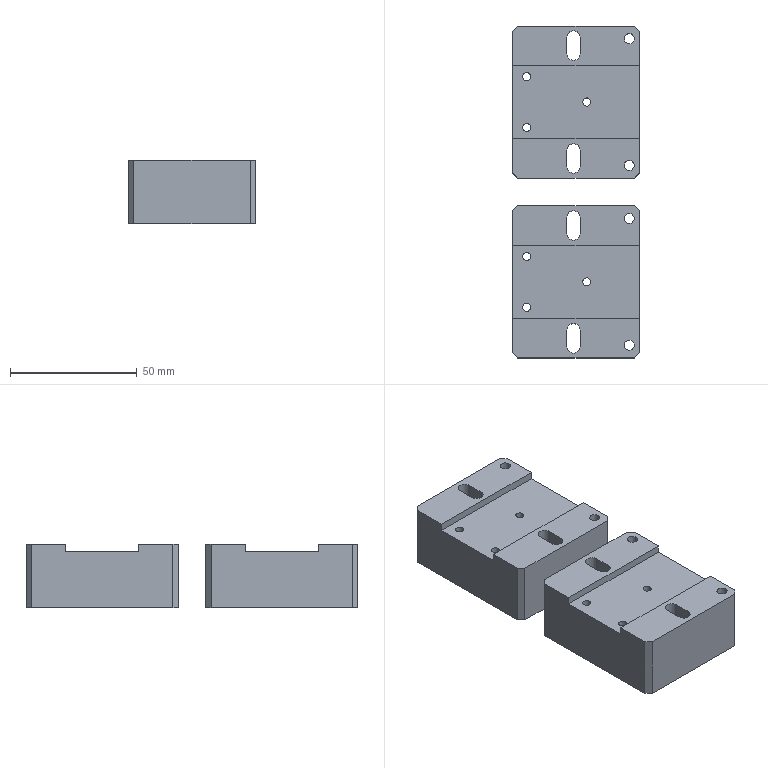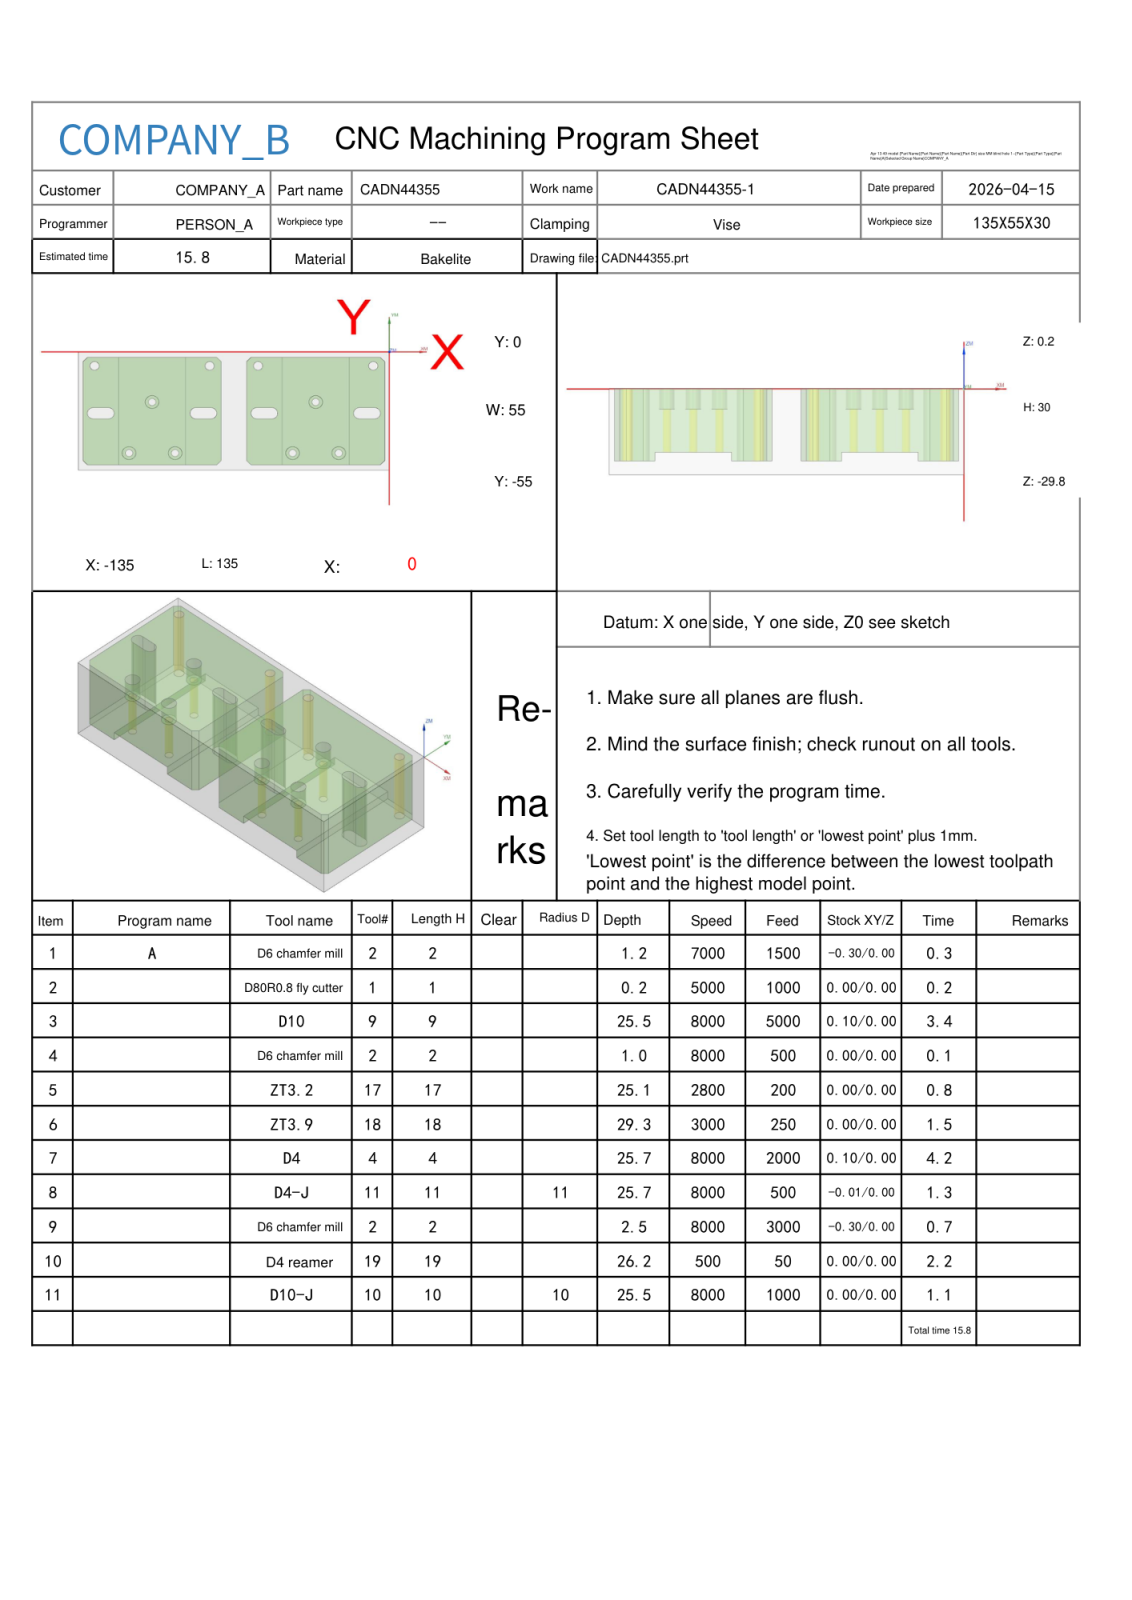NC program | NX | posted by the shop | part box 50 x 131 x 25 mm
Lines 1280 to 2096 of 5183:
N7 T04 M06
(D4  D=4. R=0. H=04 ce=0.10 di=0.10)
G00 G90 G54 X-125.275 Y-29. M03 S6000
G43 H04 Z20.
M08
Z.5
G01 X-122.05 Z.45 F2000.
G03 X-121.55 Y-28.5 Z.438 I0.0 J.5
X-122.05 Y-28. Z.426 I-.5 J0.0
G01 X-128.5 Z.326
G03 X-129. Y-28.5 Z.314 I0.0 J-.5
X-128.5 Y-29. Z.302 I.5 J0.0
G01 X-122.05 Z.203
G03 X-121.55 Y-28.5 Z.19 I0.0 J.5
X-122.05 Y-28. Z.178 I-.5 J0.0
G01 X-128.5 Z.079
G03 X-129. Y-28.5 Z.067 I0.0 J-.5
X-128.5 Y-29. Z.055 I.5 J0.0
G01 X-122.05 Z-.045
G03 X-121.55 Y-28.5 Z-.057 I0.0 J.5
X-122.05 Y-28. Z-.069 I-.5 J0.0
G01 X-128.5 Z-.169
G03 X-129. Y-28.5 Z-.181 I0.0 J-.5
X-128.5 Y-29. Z-.193 I.5 J0.0
G01 X-122.05 Z-.293
G03 X-121.55 Y-28.5 Z-.305 I0.0 J.5
X-122.05 Y-28. Z-.317 I-.5 J0.0
G01 X-128.5 Z-.416
G03 X-129. Y-28.5 Z-.429 I0.0 J-.5
X-128.5 Y-29. Z-.441 I.5 J0.0
G01 X-122.05 Z-.54
G03 X-121.55 Y-28.5 Z-.552 I0.0 J.5
X-122.05 Y-28. Z-.565 I-.5 J0.0
G01 X-128.5 Z-.664
G03 X-129. Y-28.5 Z-.676 I0.0 J-.5
X-128.5 Y-29. Z-.688 I.5 J0.0
G01 X-122.05 Z-.788
G03 X-121.55 Y-28.5 Z-.8 I0.0 J.5
X-122.05 Y-28. Z-.812 I-.5 J0.0
G01 X-128.5 Z-.912
G03 X-129. Y-28.5 Z-.924 I0.0 J-.5
X-128.5 Y-29. Z-.936 I.5 J0.0
G01 X-122.05 Z-1.035
G03 X-121.55 Y-28.5 Z-1.048 I0.0 J.5
X-122.05 Y-28. Z-1.06 I-.5 J0.0
G01 X-128.5 Z-1.159
G03 X-129. Y-28.5 Z-1.171 I0.0 J-.5
X-128.5 Y-29. Z-1.184 I.5 J0.0
G01 X-122.05 Z-1.283
G03 X-121.55 Y-28.5 Z-1.295 I0.0 J.5
X-122.05 Y-28. Z-1.307 I-.5 J0.0
G01 X-128.5 Z-1.407
G03 X-129. Y-28.5 Z-1.419 I0.0 J-.5
X-128.5 Y-29. Z-1.431 I.5 J0.0
G01 X-122.05 Z-1.531
G03 X-121.55 Y-28.5 Z-1.543 I0.0 J.5
X-122.05 Y-28. Z-1.555 I-.5 J0.0
G01 X-128.5 Z-1.655
G03 X-129. Y-28.5 Z-1.667 I0.0 J-.5
X-128.5 Y-29. Z-1.679 I.5 J0.0
G01 X-122.05 Z-1.778
G03 X-121.55 Y-28.5 Z-1.79 I0.0 J.5
X-122.05 Y-28. Z-1.803 I-.5 J0.0
G01 X-128.5 Z-1.902
G03 X-129. Y-28.5 Z-1.914 I0.0 J-.5
X-128.5 Y-29. Z-1.926 I.5 J0.0
G01 X-122.05 Z-2.026
G03 X-121.55 Y-28.5 Z-2.038 I0.0 J.5
X-122.05 Y-28. Z-2.05 I-.5 J0.0
G01 X-128.5 Z-2.15
G03 X-129. Y-28.5 Z-2.162 I0.0 J-.5
X-128.5 Y-29. Z-2.174 I.5 J0.0
G01 X-122.05 Z-2.274
G03 X-121.55 Y-28.5 Z-2.286 I0.0 J.5
X-122.05 Y-28. Z-2.298 I-.5 J0.0
G01 X-128.5 Z-2.397
G03 X-129. Y-28.5 Z-2.41 I0.0 J-.5
X-128.5 Y-29. Z-2.422 I.5 J0.0
G01 X-122.05 Z-2.521
G03 X-121.55 Y-28.5 Z-2.533 I0.0 J.5
X-122.05 Y-28. Z-2.545 I-.5 J0.0
G01 X-128.5 Z-2.645
G03 X-129. Y-28.5 Z-2.657 I0.0 J-.5
X-128.5 Y-29. Z-2.669 I.5 J0.0
G01 X-122.05 Z-2.769
G03 X-121.55 Y-28.5 Z-2.781 I0.0 J.5
X-122.05 Y-28. Z-2.793 I-.5 J0.0
G01 X-128.5 Z-2.893
G03 X-129. Y-28.5 Z-2.905 I0.0 J-.5
X-128.5 Y-29. Z-2.917 I.5 J0.0
G01 X-122.05 Z-3.016
G03 X-121.55 Y-28.5 Z-3.029 I0.0 J.5
X-122.05 Y-28. Z-3.041 I-.5 J0.0
G01 X-128.5 Z-3.14
G03 X-129. Y-28.5 Z-3.152 I0.0 J-.5
X-128.5 Y-29. Z-3.165 I.5 J0.0
G01 X-122.05 Z-3.264
G03 X-121.55 Y-28.5 Z-3.276 I0.0 J.5
X-122.05 Y-28. Z-3.288 I-.5 J0.0
G01 X-128.5 Z-3.388
G03 X-129. Y-28.5 Z-3.4 I0.0 J-.5
X-128.5 Y-29. Z-3.412 I.5 J0.0
G01 X-122.05 Z-3.512
G03 X-121.55 Y-28.5 Z-3.524 I0.0 J.5
X-122.05 Y-28. Z-3.536 I-.5 J0.0
G01 X-128.5 Z-3.635
G03 X-129. Y-28.5 Z-3.648 I0.0 J-.5
X-128.5 Y-29. Z-3.66 I.5 J0.0
G01 X-122.05 Z-3.759
G03 X-121.55 Y-28.5 Z-3.771 I0.0 J.5
X-122.05 Y-28. Z-3.784 I-.5 J0.0
G01 X-128.5 Z-3.883
G03 X-129. Y-28.5 Z-3.895 I0.0 J-.5
X-128.5 Y-29. Z-3.907 I.5 J0.0
G01 X-122.05 Z-4.007
G03 X-121.55 Y-28.5 Z-4.019 I0.0 J.5
X-122.05 Y-28. Z-4.031 I-.5 J0.0
G01 X-128.5 Z-4.131
G03 X-129. Y-28.5 Z-4.143 I0.0 J-.5
X-128.5 Y-29. Z-4.155 I.5 J0.0
G01 X-122.05 Z-4.255
G03 X-121.55 Y-28.5 Z-4.267 I0.0 J.5
X-122.05 Y-28. Z-4.279 I-.5 J0.0
G01 X-128.5 Z-4.378
G03 X-129. Y-28.5 Z-4.39 I0.0 J-.5
X-128.5 Y-29. Z-4.403 I.5 J0.0
G01 X-122.05 Z-4.502
G03 X-121.55 Y-28.5 Z-4.514 I0.0 J.5
X-122.05 Y-28. Z-4.526 I-.5 J0.0
G01 X-128.5 Z-4.626
G03 X-129. Y-28.5 Z-4.638 I0.0 J-.5
X-128.5 Y-29. Z-4.65 I.5 J0.0
G01 X-122.05 Z-4.75
G03 X-121.55 Y-28.5 Z-4.762 I0.0 J.5
X-122.05 Y-28. Z-4.774 I-.5 J0.0
G01 X-128.5 Z-4.874
G03 X-129. Y-28.5 Z-4.886 I0.0 J-.5
X-128.5 Y-29. Z-4.898 I.5 J0.0
G01 X-122.05 Z-4.997
G03 X-121.55 Y-28.5 Z-5.01 I0.0 J.5
X-122.05 Y-28. Z-5.022 I-.5 J0.0
G01 X-128.5 Z-5.121
G03 X-129. Y-28.5 Z-5.133 I0.0 J-.5
X-128.5 Y-29. Z-5.145 I.5 J0.0
G01 X-122.05 Z-5.245
G03 X-121.55 Y-28.5 Z-5.257 I0.0 J.5
X-122.05 Y-28. Z-5.269 I-.5 J0.0
G01 X-128.5 Z-5.369
G03 X-129. Y-28.5 Z-5.381 I0.0 J-.5
X-128.5 Y-29. Z-5.393 I.5 J0.0
G01 X-122.05 Z-5.493
G03 X-121.55 Y-28.5 Z-5.505 I0.0 J.5
X-122.05 Y-28. Z-5.517 I-.5 J0.0
G01 X-128.5 Z-5.616
G03 X-129. Y-28.5 Z-5.629 I0.0 J-.5
X-128.5 Y-29. Z-5.641 I.5 J0.0
G01 X-122.05 Z-5.74
G03 X-121.55 Y-28.5 Z-5.752 I0.0 J.5
X-122.05 Y-28. Z-5.765 I-.5 J0.0
G01 X-128.5 Z-5.864
G03 X-129. Y-28.5 Z-5.876 I0.0 J-.5
X-128.5 Y-29. Z-5.888 I.5 J0.0
G01 X-122.05 Z-5.988
G03 X-121.55 Y-28.5 Z-6. I0.0 J.5
X-122.05 Y-28. Z-6.012 I-.5 J0.0
G01 X-128.5 Z-6.112
G03 X-129. Y-28.5 Z-6.124 I0.0 J-.5
X-128.5 Y-29. Z-6.136 I.5 J0.0
G01 X-122.05 Z-6.235
G03 X-121.55 Y-28.5 Z-6.248 I0.0 J.5
X-122.05 Y-28. Z-6.26 I-.5 J0.0
G01 X-128.5 Z-6.359
G03 X-129. Y-28.5 Z-6.371 I0.0 J-.5
X-128.5 Y-29. Z-6.384 I.5 J0.0
G01 X-122.05 Z-6.483
G03 X-121.55 Y-28.5 Z-6.495 I0.0 J.5
X-122.05 Y-28. Z-6.507 I-.5 J0.0
G01 X-128.5 Z-6.607
G03 X-129. Y-28.5 Z-6.619 I0.0 J-.5
X-128.5 Y-29. Z-6.631 I.5 J0.0
G01 X-122.05 Z-6.731
G03 X-121.55 Y-28.5 Z-6.743 I0.0 J.5
X-122.05 Y-28. Z-6.755 I-.5 J0.0
G01 X-128.5 Z-6.855
G03 X-129. Y-28.5 Z-6.867 I0.0 J-.5
X-128.5 Y-29. Z-6.879 I.5 J0.0
G01 X-122.05 Z-6.978
G03 X-121.55 Y-28.5 Z-6.99 I0.0 J.5
X-122.05 Y-28. Z-7.003 I-.5 J0.0
G01 X-128.5 Z-7.102
G03 X-129. Y-28.5 Z-7.114 I0.0 J-.5
X-128.5 Y-29. Z-7.126 I.5 J0.0
G01 X-122.05 Z-7.226
G03 X-121.55 Y-28.5 Z-7.238 I0.0 J.5
X-122.05 Y-28. Z-7.25 I-.5 J0.0
G01 X-128.5 Z-7.35
G03 X-129. Y-28.5 Z-7.362 I0.0 J-.5
X-128.5 Y-29. Z-7.374 I.5 J0.0
G01 X-122.05 Z-7.474
G03 X-121.55 Y-28.5 Z-7.486 I0.0 J.5
X-122.05 Y-28. Z-7.498 I-.5 J0.0
G01 X-128.5 Z-7.597
G03 X-129. Y-28.5 Z-7.61 I0.0 J-.5
X-128.5 Y-29. Z-7.622 I.5 J0.0
G01 X-122.05 Z-7.721
G03 X-121.55 Y-28.5 Z-7.733 I0.0 J.5
X-122.05 Y-28. Z-7.745 I-.5 J0.0
G01 X-128.5 Z-7.845
G03 X-129. Y-28.5 Z-7.857 I0.0 J-.5
X-128.5 Y-29. Z-7.869 I.5 J0.0
G01 X-122.05 Z-7.969
G03 X-121.55 Y-28.5 Z-7.981 I0.0 J.5
X-122.05 Y-28. Z-7.993 I-.5 J0.0
G01 X-128.5 Z-8.093
G03 X-129. Y-28.5 Z-8.105 I0.0 J-.5
X-128.5 Y-29. Z-8.117 I.5 J0.0
G01 X-122.05 Z-8.216
G03 X-121.55 Y-28.5 Z-8.229 I0.0 J.5
X-122.05 Y-28. Z-8.241 I-.5 J0.0
G01 X-128.5 Z-8.34
G03 X-129. Y-28.5 Z-8.352 I0.0 J-.5
X-128.5 Y-29. Z-8.365 I.5 J0.0
G01 X-122.05 Z-8.464
G03 X-121.55 Y-28.5 Z-8.476 I0.0 J.5
X-122.05 Y-28. Z-8.488 I-.5 J0.0
G01 X-128.5 Z-8.588
G03 X-129. Y-28.5 Z-8.6 I0.0 J-.5
X-128.5 Y-29. Z-8.612 I.5 J0.0
G01 X-122.05 Z-8.712
G03 X-121.55 Y-28.5 Z-8.724 I0.0 J.5
X-122.05 Y-28. Z-8.736 I-.5 J0.0
G01 X-128.5 Z-8.835
G03 X-129. Y-28.5 Z-8.848 I0.0 J-.5
X-128.5 Y-29. Z-8.86 I.5 J0.0
G01 X-122.05 Z-8.959
G03 X-121.55 Y-28.5 Z-8.971 I0.0 J.5
X-122.05 Y-28. Z-8.984 I-.5 J0.0
G01 X-128.5 Z-9.083
G03 X-129. Y-28.5 Z-9.095 I0.0 J-.5
X-128.5 Y-29. Z-9.107 I.5 J0.0
G01 X-122.05 Z-9.207
G03 X-121.55 Y-28.5 Z-9.219 I0.0 J.5
X-122.05 Y-28. Z-9.231 I-.5 J0.0
G01 X-128.5 Z-9.331
G03 X-129. Y-28.5 Z-9.343 I0.0 J-.5
X-128.5 Y-29. Z-9.355 I.5 J0.0
G01 X-122.05 Z-9.455
G03 X-121.55 Y-28.5 Z-9.467 I0.0 J.5
X-122.05 Y-28. Z-9.479 I-.5 J0.0
G01 X-128.5 Z-9.578
G03 X-129. Y-28.5 Z-9.59 I0.0 J-.5
X-128.5 Y-29. Z-9.603 I.5 J0.0
G01 X-122.05 Z-9.702
G03 X-121.55 Y-28.5 Z-9.714 I0.0 J.5
X-122.05 Y-28. Z-9.726 I-.5 J0.0
G01 X-128.5 Z-9.826
G03 X-129. Y-28.5 Z-9.838 I0.0 J-.5
X-128.5 Y-29. Z-9.85 I.5 J0.0
G01 X-122.05 Z-9.95
G03 X-121.55 Y-28.5 Z-9.962 I0.0 J.5
X-122.05 Y-28. Z-9.974 I-.5 J0.0
G01 X-128.5 Z-10.074
G03 X-129. Y-28.5 Z-10.086 I0.0 J-.5
X-128.5 Y-29. Z-10.098 I.5 J0.0
G01 X-122.05 Z-10.197
G03 X-121.55 Y-28.5 Z-10.21 I0.0 J.5
X-122.05 Y-28. Z-10.222 I-.5 J0.0
G01 X-128.5 Z-10.321
G03 X-129. Y-28.5 Z-10.333 I0.0 J-.5
X-128.5 Y-29. Z-10.345 I.5 J0.0
G01 X-122.05 Z-10.445
G03 X-121.55 Y-28.5 Z-10.457 I0.0 J.5
X-122.05 Y-28. Z-10.469 I-.5 J0.0
G01 X-128.5 Z-10.569
G03 X-129. Y-28.5 Z-10.581 I0.0 J-.5
X-128.5 Y-29. Z-10.593 I.5 J0.0
G01 X-122.05 Z-10.693
G03 X-121.55 Y-28.5 Z-10.705 I0.0 J.5
X-122.05 Y-28. Z-10.717 I-.5 J0.0
G01 X-128.5 Z-10.816
G03 X-129. Y-28.5 Z-10.829 I0.0 J-.5
X-128.5 Y-29. Z-10.841 I.5 J0.0
G01 X-122.05 Z-10.94
G03 X-121.55 Y-28.5 Z-10.952 I0.0 J.5
X-122.05 Y-28. Z-10.965 I-.5 J0.0
G01 X-128.5 Z-11.064
G03 X-129. Y-28.5 Z-11.076 I0.0 J-.5
X-128.5 Y-29. Z-11.088 I.5 J0.0
G01 X-122.05 Z-11.188
G03 X-121.55 Y-28.5 Z-11.2 I0.0 J.5
X-122.05 Y-28. Z-11.212 I-.5 J0.0
G01 X-128.5 Z-11.312
G03 X-129. Y-28.5 Z-11.324 I0.0 J-.5
X-128.5 Y-29. Z-11.336 I.5 J0.0
G01 X-122.05 Z-11.435
G03 X-121.55 Y-28.5 Z-11.448 I0.0 J.5
X-122.05 Y-28. Z-11.46 I-.5 J0.0
G01 X-128.5 Z-11.559
G03 X-129. Y-28.5 Z-11.571 I0.0 J-.5
X-128.5 Y-29. Z-11.584 I.5 J0.0
G01 X-122.05 Z-11.683
G03 X-121.55 Y-28.5 Z-11.695 I0.0 J.5
X-122.05 Y-28. Z-11.707 I-.5 J0.0
G01 X-128.5 Z-11.807
G03 X-129. Y-28.5 Z-11.819 I0.0 J-.5
X-128.5 Y-29. Z-11.831 I.5 J0.0
G01 X-122.05 Z-11.931
G03 X-121.55 Y-28.5 Z-11.943 I0.0 J.5
X-122.05 Y-28. Z-11.955 I-.5 J0.0
G01 X-128.5 Z-12.055
G03 X-129. Y-28.5 Z-12.067 I0.0 J-.5
X-128.5 Y-29. Z-12.079 I.5 J0.0
G01 X-122.05 Z-12.178
G03 X-121.55 Y-28.5 Z-12.19 I0.0 J.5
X-122.05 Y-28. Z-12.203 I-.5 J0.0
G01 X-128.5 Z-12.302
G03 X-129. Y-28.5 Z-12.314 I0.0 J-.5
X-128.5 Y-29. Z-12.326 I.5 J0.0
G01 X-122.05 Z-12.426
G03 X-121.55 Y-28.5 Z-12.438 I0.0 J.5
X-122.05 Y-28. Z-12.45 I-.5 J0.0
G01 X-128.5 Z-12.55
G03 X-129. Y-28.5 Z-12.562 I0.0 J-.5
X-128.5 Y-29. Z-12.574 I.5 J0.0
G01 X-122.05 Z-12.674
G03 X-121.55 Y-28.5 Z-12.686 I0.0 J.5
X-122.05 Y-28. Z-12.698 I-.5 J0.0
G01 X-128.5 Z-12.797
G03 X-129. Y-28.5 Z-12.81 I0.0 J-.5
X-128.5 Y-29. Z-12.822 I.5 J0.0
G01 X-122.05 Z-12.921
G03 X-121.55 Y-28.5 Z-12.933 I0.0 J.5
X-122.05 Y-28. Z-12.945 I-.5 J0.0
G01 X-128.5 Z-13.045
G03 X-129. Y-28.5 Z-13.057 I0.0 J-.5
X-128.5 Y-29. Z-13.069 I.5 J0.0
G01 X-122.05 Z-13.169
G03 X-121.55 Y-28.5 Z-13.181 I0.0 J.5
X-122.05 Y-28. Z-13.193 I-.5 J0.0
G01 X-128.5 Z-13.293
G03 X-129. Y-28.5 Z-13.305 I0.0 J-.5
X-128.5 Y-29. Z-13.317 I.5 J0.0
G01 X-122.05 Z-13.416
G03 X-121.55 Y-28.5 Z-13.429 I0.0 J.5
X-122.05 Y-28. Z-13.441 I-.5 J0.0
G01 X-128.5 Z-13.54
G03 X-129. Y-28.5 Z-13.552 I0.0 J-.5
X-128.5 Y-29. Z-13.565 I.5 J0.0
G01 X-122.05 Z-13.664
G03 X-121.55 Y-28.5 Z-13.676 I0.0 J.5
X-122.05 Y-28. Z-13.688 I-.5 J0.0
G01 X-128.5 Z-13.788
G03 X-129. Y-28.5 Z-13.8 I0.0 J-.5
X-128.5 Y-29. Z-13.812 I.5 J0.0
G01 X-122.05 Z-13.912
G03 X-121.55 Y-28.5 Z-13.924 I0.0 J.5
X-122.05 Y-28. Z-13.936 I-.5 J0.0
G01 X-128.5 Z-14.035
G03 X-129. Y-28.5 Z-14.048 I0.0 J-.5
X-128.5 Y-29. Z-14.06 I.5 J0.0
G01 X-122.05 Z-14.159
G03 X-121.55 Y-28.5 Z-14.171 I0.0 J.5
X-122.05 Y-28. Z-14.184 I-.5 J0.0
G01 X-128.5 Z-14.283
G03 X-129. Y-28.5 Z-14.295 I0.0 J-.5
X-128.5 Y-29. Z-14.307 I.5 J0.0
G01 X-122.05 Z-14.407
G03 X-121.55 Y-28.5 Z-14.419 I0.0 J.5
X-122.05 Y-28. Z-14.431 I-.5 J0.0
G01 X-128.5 Z-14.531
G03 X-129. Y-28.5 Z-14.543 I0.0 J-.5
X-128.5 Y-29. Z-14.555 I.5 J0.0
G01 X-122.05 Z-14.655
G03 X-121.55 Y-28.5 Z-14.667 I0.0 J.5
X-122.05 Y-28. Z-14.679 I-.5 J0.0
G01 X-128.5 Z-14.778
G03 X-129. Y-28.5 Z-14.79 I0.0 J-.5
X-128.5 Y-29. Z-14.803 I.5 J0.0
G01 X-122.05 Z-14.902
G03 X-121.55 Y-28.5 Z-14.914 I0.0 J.5
X-122.05 Y-28. Z-14.926 I-.5 J0.0
G01 X-128.5 Z-15.026
G03 X-129. Y-28.5 Z-15.038 I0.0 J-.5
X-128.5 Y-29. Z-15.05 I.5 J0.0
G01 X-122.05 Z-15.15
G03 X-121.55 Y-28.5 Z-15.162 I0.0 J.5
X-122.05 Y-28. Z-15.174 I-.5 J0.0
G01 X-128.5 Z-15.274
G03 X-129. Y-28.5 Z-15.286 I0.0 J-.5
X-128.5 Y-29. Z-15.298 I.5 J0.0
G01 X-122.05 Z-15.397
G03 X-121.55 Y-28.5 Z-15.41 I0.0 J.5
X-122.05 Y-28. Z-15.422 I-.5 J0.0
G01 X-128.5 Z-15.521
G03 X-129. Y-28.5 Z-15.533 I0.0 J-.5
X-128.5 Y-29. Z-15.545 I.5 J0.0
G01 X-122.05 Z-15.645
G03 X-121.55 Y-28.5 Z-15.657 I0.0 J.5
X-122.05 Y-28. Z-15.669 I-.5 J0.0
G01 X-128.5 Z-15.769
G03 X-129. Y-28.5 Z-15.781 I0.0 J-.5
X-128.5 Y-29. Z-15.793 I.5 J0.0
G01 X-122.05 Z-15.893
G03 X-121.55 Y-28.5 Z-15.905 I0.0 J.5
X-122.05 Y-28. Z-15.917 I-.5 J0.0
G01 X-128.5 Z-16.016
G03 X-129. Y-28.5 Z-16.029 I0.0 J-.5
X-128.5 Y-29. Z-16.041 I.5 J0.0
G01 X-122.05 Z-16.14
G03 X-121.55 Y-28.5 Z-16.152 I0.0 J.5
X-122.05 Y-28. Z-16.165 I-.5 J0.0
G01 X-128.5 Z-16.264
G03 X-129. Y-28.5 Z-16.276 I0.0 J-.5
X-128.5 Y-29. Z-16.288 I.5 J0.0
G01 X-122.05 Z-16.388
G03 X-121.55 Y-28.5 Z-16.4 I0.0 J.5
X-122.05 Y-28. Z-16.412 I-.5 J0.0
G01 X-128.5 Z-16.512
G03 X-129. Y-28.5 Z-16.524 I0.0 J-.5
X-128.5 Y-29. Z-16.536 I.5 J0.0
G01 X-122.05 Z-16.635
G03 X-121.55 Y-28.5 Z-16.648 I0.0 J.5
X-122.05 Y-28. Z-16.66 I-.5 J0.0
G01 X-128.5 Z-16.759
G03 X-129. Y-28.5 Z-16.771 I0.0 J-.5
X-128.5 Y-29. Z-16.784 I.5 J0.0
G01 X-122.05 Z-16.883
G03 X-121.55 Y-28.5 Z-16.895 I0.0 J.5
X-122.05 Y-28. Z-16.907 I-.5 J0.0
G01 X-128.5 Z-17.007
G03 X-129. Y-28.5 Z-17.019 I0.0 J-.5
X-128.5 Y-29. Z-17.031 I.5 J0.0
G01 X-122.05 Z-17.131
G03 X-121.55 Y-28.5 Z-17.143 I0.0 J.5
X-122.05 Y-28. Z-17.155 I-.5 J0.0
G01 X-128.5 Z-17.255
G03 X-129. Y-28.5 Z-17.267 I0.0 J-.5
X-128.5 Y-29. Z-17.279 I.5 J0.0
G01 X-122.05 Z-17.378
G03 X-121.55 Y-28.5 Z-17.39 I0.0 J.5
X-122.05 Y-28. Z-17.403 I-.5 J0.0
G01 X-128.5 Z-17.502
G03 X-129. Y-28.5 Z-17.514 I0.0 J-.5
X-128.5 Y-29. Z-17.526 I.5 J0.0
G01 X-122.05 Z-17.626
G03 X-121.55 Y-28.5 Z-17.638 I0.0 J.5
X-122.05 Y-28. Z-17.65 I-.5 J0.0
G01 X-128.5 Z-17.75
G03 X-129. Y-28.5 Z-17.762 I0.0 J-.5
X-128.5 Y-29. Z-17.774 I.5 J0.0
G01 X-122.05 Z-17.874
G03 X-121.55 Y-28.5 Z-17.886 I0.0 J.5
X-122.05 Y-28. Z-17.898 I-.5 J0.0
G01 X-128.5 Z-17.997
G03 X-129. Y-28.5 Z-18.01 I0.0 J-.5
X-128.5 Y-29. Z-18.022 I.5 J0.0
G01 X-122.05 Z-18.121
G03 X-121.55 Y-28.5 Z-18.133 I0.0 J.5
X-122.05 Y-28. Z-18.145 I-.5 J0.0
G01 X-128.5 Z-18.245
G03 X-129. Y-28.5 Z-18.257 I0.0 J-.5
X-128.5 Y-29. Z-18.269 I.5 J0.0
G01 X-122.05 Z-18.369
G03 X-121.55 Y-28.5 Z-18.381 I0.0 J.5
X-122.05 Y-28. Z-18.393 I-.5 J0.0
G01 X-128.5 Z-18.493
G03 X-129. Y-28.5 Z-18.505 I0.0 J-.5
X-128.5 Y-29. Z-18.517 I.5 J0.0
G01 X-122.05 Z-18.616
G03 X-121.55 Y-28.5 Z-18.629 I0.0 J.5
X-122.05 Y-28. Z-18.641 I-.5 J0.0
G01 X-128.5 Z-18.74
G03 X-129. Y-28.5 Z-18.752 I0.0 J-.5
X-128.5 Y-29. Z-18.765 I.5 J0.0
G01 X-122.05 Z-18.864
G03 X-121.55 Y-28.5 Z-18.876 I0.0 J.5
X-122.05 Y-28. Z-18.888 I-.5 J0.0
G01 X-128.5 Z-18.988
G03 X-129. Y-28.5 Z-19. I0.0 J-.5
X-128.5 Y-29. Z-19.012 I.5 J0.0
G01 X-122.05 Z-19.112
G03 X-121.55 Y-28.5 Z-19.124 I0.0 J.5
X-122.05 Y-28. Z-19.136 I-.5 J0.0
G01 X-128.5 Z-19.235
G03 X-129. Y-28.5 Z-19.248 I0.0 J-.5
X-128.5 Y-29. Z-19.26 I.5 J0.0
G01 X-122.05 Z-19.359
G03 X-121.55 Y-28.5 Z-19.371 I0.0 J.5
X-122.05 Y-28. Z-19.384 I-.5 J0.0
G01 X-128.5 Z-19.483
G03 X-129. Y-28.5 Z-19.495 I0.0 J-.5
X-128.5 Y-29. Z-19.507 I.5 J0.0
G01 X-122.05 Z-19.607
G03 X-121.55 Y-28.5 Z-19.619 I0.0 J.5
X-122.05 Y-28. Z-19.631 I-.5 J0.0
G01 X-128.5 Z-19.731
G03 X-129. Y-28.5 Z-19.743 I0.0 J-.5
X-128.5 Y-29. Z-19.755 I.5 J0.0
G01 X-122.05 Z-19.855
G03 X-121.55 Y-28.5 Z-19.867 I0.0 J.5
X-122.05 Y-28. Z-19.879 I-.5 J0.0
G01 X-128.5 Z-19.978
G03 X-129. Y-28.5 Z-19.99 I0.0 J-.5
X-128.5 Y-29. Z-20.003 I.5 J0.0
G01 X-122.05 Z-20.102
G03 X-121.55 Y-28.5 Z-20.114 I0.0 J.5
X-122.05 Y-28. Z-20.126 I-.5 J0.0
G01 X-128.5 Z-20.226
G03 X-129. Y-28.5 Z-20.238 I0.0 J-.5
X-128.5 Y-29. Z-20.25 I.5 J0.0
G01 X-122.05 Z-20.35
G03 X-121.55 Y-28.5 Z-20.362 I0.0 J.5
X-122.05 Y-28. Z-20.374 I-.5 J0.0
G01 X-128.5 Z-20.474
G03 X-129. Y-28.5 Z-20.486 I0.0 J-.5
X-128.5 Y-29. Z-20.498 I.5 J0.0
G01 X-122.05 Z-20.597
G03 X-121.55 Y-28.5 Z-20.61 I0.0 J.5
X-122.05 Y-28. Z-20.622 I-.5 J0.0
G01 X-128.5 Z-20.721
G03 X-129. Y-28.5 Z-20.733 I0.0 J-.5
X-128.5 Y-29. Z-20.745 I.5 J0.0
G01 X-122.05 Z-20.845
G03 X-121.55 Y-28.5 Z-20.857 I0.0 J.5
X-122.05 Y-28. Z-20.869 I-.5 J0.0
G01 X-128.5 Z-20.969
G03 X-129. Y-28.5 Z-20.981 I0.0 J-.5
X-128.5 Y-29. Z-20.993 I.5 J0.0
G01 X-122.05 Z-21.093
G03 X-121.55 Y-28.5 Z-21.105 I0.0 J.5
X-122.05 Y-28. Z-21.117 I-.5 J0.0
G01 X-128.5 Z-21.216
G03 X-129. Y-28.5 Z-21.229 I0.0 J-.5
X-128.5 Y-29. Z-21.241 I.5 J0.0
G01 X-122.05 Z-21.34
G03 X-121.55 Y-28.5 Z-21.352 I0.0 J.5
X-122.05 Y-28. Z-21.365 I-.5 J0.0
G01 X-128.5 Z-21.464
G03 X-129. Y-28.5 Z-21.476 I0.0 J-.5
X-128.5 Y-29. Z-21.488 I.5 J0.0
G01 X-122.05 Z-21.588
G03 X-121.55 Y-28.5 Z-21.6 I0.0 J.5
X-122.05 Y-28. Z-21.612 I-.5 J0.0
G01 X-128.5 Z-21.712
G03 X-129. Y-28.5 Z-21.724 I0.0 J-.5
X-128.5 Y-29. Z-21.736 I.5 J0.0
G01 X-122.05 Z-21.835
G03 X-121.55 Y-28.5 Z-21.848 I0.0 J.5
X-122.05 Y-28. Z-21.86 I-.5 J0.0
G01 X-128.5 Z-21.959
G03 X-129. Y-28.5 Z-21.971 I0.0 J-.5
X-128.5 Y-29. Z-21.984 I.5 J0.0
G01 X-122.05 Z-22.083
G03 X-121.55 Y-28.5 Z-22.095 I0.0 J.5
X-122.05 Y-28. Z-22.107 I-.5 J0.0
G01 X-128.5 Z-22.207
G03 X-129. Y-28.5 Z-22.219 I0.0 J-.5
X-128.5 Y-29. Z-22.231 I.5 J0.0
G01 X-122.05 Z-22.331
G03 X-121.55 Y-28.5 Z-22.343 I0.0 J.5
X-122.05 Y-28. Z-22.355 I-.5 J0.0
G01 X-128.5 Z-22.455
G03 X-129. Y-28.5 Z-22.467 I0.0 J-.5
X-128.5 Y-29. Z-22.479 I.5 J0.0
G01 X-122.05 Z-22.578
G03 X-121.55 Y-28.5 Z-22.59 I0.0 J.5
X-122.05 Y-28. Z-22.603 I-.5 J0.0
G01 X-128.5 Z-22.702
G03 X-129. Y-28.5 Z-22.714 I0.0 J-.5
X-128.5 Y-29. Z-22.726 I.5 J0.0
G01 X-122.05 Z-22.826
G03 X-121.55 Y-28.5 Z-22.838 I0.0 J.5
X-122.05 Y-28. Z-22.85 I-.5 J0.0
G01 X-128.5 Z-22.95
G03 X-129. Y-28.5 Z-22.962 I0.0 J-.5
X-128.5 Y-29. Z-22.974 I.5 J0.0
G01 X-122.05 Z-23.074
G03 X-121.55 Y-28.5 Z-23.086 I0.0 J.5
X-122.05 Y-28. Z-23.098 I-.5 J0.0
G01 X-128.5 Z-23.197
G03 X-129. Y-28.5 Z-23.21 I0.0 J-.5
X-128.5 Y-29. Z-23.222 I.5 J0.0
G01 X-122.05 Z-23.321
G03 X-121.55 Y-28.5 Z-23.333 I0.0 J.5
X-122.05 Y-28. Z-23.345 I-.5 J0.0
G01 X-128.5 Z-23.445
G03 X-129. Y-28.5 Z-23.457 I0.0 J-.5
X-128.5 Y-29. Z-23.469 I.5 J0.0
G01 X-122.05 Z-23.569
G03 X-121.55 Y-28.5 Z-23.581 I0.0 J.5
X-122.05 Y-28. Z-23.593 I-.5 J0.0
G01 X-128.5 Z-23.693
G03 X-129. Y-28.5 Z-23.705 I0.0 J-.5
X-128.5 Y-29. Z-23.717 I.5 J0.0
G01 X-122.05 Z-23.816
G03 X-121.55 Y-28.5 Z-23.829 I0.0 J.5
X-122.05 Y-28. Z-23.841 I-.5 J0.0
G01 X-128.5 Z-23.94
G03 X-129. Y-28.5 Z-23.952 I0.0 J-.5
X-128.5 Y-29. Z-23.965 I.5 J0.0
G01 X-122.05 Z-24.064
G03 X-121.55 Y-28.5 Z-24.076 I0.0 J.5
X-122.05 Y-28. Z-24.088 I-.5 J0.0
G01 X-128.5 Z-24.188
G03 X-129. Y-28.5 Z-24.2 I0.0 J-.5
X-128.5 Y-29. Z-24.212 I.5 J0.0
G01 X-122.05 Z-24.312
G03 X-121.55 Y-28.5 Z-24.324 I0.0 J.5
X-122.05 Y-28. Z-24.336 I-.5 J0.0
G01 X-128.5 Z-24.435
G03 X-129. Y-28.5 Z-24.448 I0.0 J-.5
X-128.5 Y-29. Z-24.46 I.5 J0.0
G01 X-122.05 Z-24.559
G03 X-121.55 Y-28.5 Z-24.571 I0.0 J.5
X-122.05 Y-28. Z-24.584 I-.5 J0.0
G01 X-128.5 Z-24.683
G03 X-129. Y-28.5 Z-24.695 I0.0 J-.5
X-128.5 Y-29. Z-24.707 I.5 J0.0
G01 X-122.05 Z-24.807
G03 X-121.55 Y-28.5 Z-24.819 I0.0 J.5
X-122.05 Y-28. Z-24.831 I-.5 J0.0
G01 X-128.5 Z-24.931
G03 X-129. Y-28.5 Z-24.943 I0.0 J-.5
X-128.5 Y-29. Z-24.955 I.5 J0.0
G01 X-122.05 Z-25.055
G03 X-121.55 Y-28.5 Z-25.067 I0.0 J.5
X-122.05 Y-28. Z-25.079 I-.5 J0.0
G01 X-128.5 Z-25.178
G03 X-129. Y-28.5 Z-25.19 I0.0 J-.5
X-128.5 Y-29. Z-25.203 I.5 J0.0
G01 X-122.05 Z-25.302
G03 X-121.55 Y-28.5 Z-25.314 I0.0 J.5
X-122.05 Y-28. Z-25.326 I-.5 J0.0
G01 X-128.5 Z-25.426
G03 X-129. Y-28.5 Z-25.438 I0.0 J-.5
X-128.5 Y-29. Z-25.45 I.5 J0.0
G01 X-125.275 Z-25.5
X-122.05
G03 X-121.55 Y-28.5 I0.0 J.5
X-122.05 Y-28. I-.5 J0.0
G01 X-128.5
G03 X-129. Y-28.5 I0.0 J-.5
X-128.5 Y-29. I.5 J0.0
G01 X-125.275
X-124.775
Z-24.5
G00 Z20.
X-80.725
Z.5
G01 X-77.5 Z.45
G03 X-77. Y-28.5 Z.438 I0.0 J.5
X-77.5 Y-28. Z.426 I-.5 J0.0
G01 X-83.95 Z.326
G03 X-84.45 Y-28.5 Z.314 I0.0 J-.5
X-83.95 Y-29. Z.302 I.5 J0.0
G01 X-77.5 Z.203
G03 X-77. Y-28.5 Z.19 I0.0 J.5
X-77.5 Y-28. Z.178 I-.5 J0.0
G01 X-83.95 Z.079
G03 X-84.45 Y-28.5 Z.067 I0.0 J-.5
X-83.95 Y-29. Z.055 I.5 J0.0
G01 X-77.5 Z-.045
G03 X-77. Y-28.5 Z-.057 I0.0 J.5
X-77.5 Y-28. Z-.069 I-.5 J0.0
G01 X-83.95 Z-.169
G03 X-84.45 Y-28.5 Z-.181 I0.0 J-.5
X-83.95 Y-29. Z-.193 I.5 J0.0
G01 X-77.5 Z-.293
G03 X-77. Y-28.5 Z-.305 I0.0 J.5
X-77.5 Y-28. Z-.317 I-.5 J0.0
G01 X-83.95 Z-.416
G03 X-84.45 Y-28.5 Z-.429 I0.0 J-.5
X-83.95 Y-29. Z-.441 I.5 J0.0
G01 X-77.5 Z-.54
G03 X-77. Y-28.5 Z-.552 I0.0 J.5
X-77.5 Y-28. Z-.565 I-.5 J0.0
G01 X-83.95 Z-.664
G03 X-84.45 Y-28.5 Z-.676 I0.0 J-.5
X-83.95 Y-29. Z-.688 I.5 J0.0
G01 X-77.5 Z-.788
G03 X-77. Y-28.5 Z-.8 I0.0 J.5
X-77.5 Y-28. Z-.812 I-.5 J0.0
G01 X-83.95 Z-.912
G03 X-84.45 Y-28.5 Z-.924 I0.0 J-.5
X-83.95 Y-29. Z-.936 I.5 J0.0
G01 X-77.5 Z-1.035
G03 X-77. Y-28.5 Z-1.048 I0.0 J.5
X-77.5 Y-28. Z-1.06 I-.5 J0.0
G01 X-83.95 Z-1.159
G03 X-84.45 Y-28.5 Z-1.171 I0.0 J-.5
X-83.95 Y-29. Z-1.184 I.5 J0.0
G01 X-77.5 Z-1.283
G03 X-77. Y-28.5 Z-1.295 I0.0 J.5
X-77.5 Y-28. Z-1.307 I-.5 J0.0
G01 X-83.95 Z-1.407
G03 X-84.45 Y-28.5 Z-1.419 I0.0 J-.5
X-83.95 Y-29. Z-1.431 I.5 J0.0
G01 X-77.5 Z-1.531
G03 X-77. Y-28.5 Z-1.543 I0.0 J.5
X-77.5 Y-28. Z-1.555 I-.5 J0.0
G01 X-83.95 Z-1.655
G03 X-84.45 Y-28.5 Z-1.667 I0.0 J-.5
X-83.95 Y-29. Z-1.679 I.5 J0.0
G01 X-77.5 Z-1.778
G03 X-77. Y-28.5 Z-1.79 I0.0 J.5
X-77.5 Y-28. Z-1.803 I-.5 J0.0
G01 X-83.95 Z-1.902
G03 X-84.45 Y-28.5 Z-1.914 I0.0 J-.5
X-83.95 Y-29. Z-1.926 I.5 J0.0
G01 X-77.5 Z-2.026
G03 X-77. Y-28.5 Z-2.038 I0.0 J.5
X-77.5 Y-28. Z-2.05 I-.5 J0.0
G01 X-83.95 Z-2.15
G03 X-84.45 Y-28.5 Z-2.162 I0.0 J-.5
X-83.95 Y-29. Z-2.174 I.5 J0.0
G01 X-77.5 Z-2.274
G03 X-77. Y-28.5 Z-2.286 I0.0 J.5
X-77.5 Y-28. Z-2.298 I-.5 J0.0
G01 X-83.95 Z-2.397
G03 X-84.45 Y-28.5 Z-2.41 I0.0 J-.5
X-83.95 Y-29. Z-2.422 I.5 J0.0
G01 X-77.5 Z-2.521
G03 X-77. Y-28.5 Z-2.533 I0.0 J.5
X-77.5 Y-28. Z-2.545 I-.5 J0.0
G01 X-83.95 Z-2.645
G03 X-84.45 Y-28.5 Z-2.657 I0.0 J-.5
X-83.95 Y-29. Z-2.669 I.5 J0.0
G01 X-77.5 Z-2.769
G03 X-77. Y-28.5 Z-2.781 I0.0 J.5
X-77.5 Y-28. Z-2.793 I-.5 J0.0
G01 X-83.95 Z-2.893
G03 X-84.45 Y-28.5 Z-2.905 I0.0 J-.5
X-83.95 Y-29. Z-2.917 I.5 J0.0
G01 X-77.5 Z-3.016
G03 X-77. Y-28.5 Z-3.029 I0.0 J.5
X-77.5 Y-28. Z-3.041 I-.5 J0.0
G01 X-83.95 Z-3.14
G03 X-84.45 Y-28.5 Z-3.152 I0.0 J-.5
X-83.95 Y-29. Z-3.165 I.5 J0.0
G01 X-77.5 Z-3.264
G03 X-77. Y-28.5 Z-3.276 I0.0 J.5
X-77.5 Y-28. Z-3.288 I-.5 J0.0
G01 X-83.95 Z-3.388
G03 X-84.45 Y-28.5 Z-3.4 I0.0 J-.5
X-83.95 Y-29. Z-3.412 I.5 J0.0
G01 X-77.5 Z-3.512
G03 X-77. Y-28.5 Z-3.524 I0.0 J.5
X-77.5 Y-28. Z-3.536 I-.5 J0.0
G01 X-83.95 Z-3.635
G03 X-84.45 Y-28.5 Z-3.648 I0.0 J-.5
X-83.95 Y-29. Z-3.66 I.5 J0.0
G01 X-77.5 Z-3.759
G03 X-77. Y-28.5 Z-3.771 I0.0 J.5
X-77.5 Y-28. Z-3.784 I-.5 J0.0
G01 X-83.95 Z-3.883
G03 X-84.45 Y-28.5 Z-3.895 I0.0 J-.5
X-83.95 Y-29. Z-3.907 I.5 J0.0
G01 X-77.5 Z-4.007
G03 X-77. Y-28.5 Z-4.019 I0.0 J.5
X-77.5 Y-28. Z-4.031 I-.5 J0.0
G01 X-83.95 Z-4.131
G03 X-84.45 Y-28.5 Z-4.143 I0.0 J-.5
X-83.95 Y-29. Z-4.155 I.5 J0.0
G01 X-77.5 Z-4.255
G03 X-77. Y-28.5 Z-4.267 I0.0 J.5
X-77.5 Y-28. Z-4.279 I-.5 J0.0
G01 X-83.95 Z-4.378
G03 X-84.45 Y-28.5 Z-4.39 I0.0 J-.5
X-83.95 Y-29. Z-4.403 I.5 J0.0
G01 X-77.5 Z-4.502
G03 X-77. Y-28.5 Z-4.514 I0.0 J.5
X-77.5 Y-28. Z-4.526 I-.5 J0.0
G01 X-83.95 Z-4.626
G03 X-84.45 Y-28.5 Z-4.638 I0.0 J-.5
X-83.95 Y-29. Z-4.65 I.5 J0.0
G01 X-77.5 Z-4.75
G03 X-77. Y-28.5 Z-4.762 I0.0 J.5
X-77.5 Y-28. Z-4.774 I-.5 J0.0
G01 X-83.95 Z-4.874
G03 X-84.45 Y-28.5 Z-4.886 I0.0 J-.5
X-83.95 Y-29. Z-4.898 I.5 J0.0
G01 X-77.5 Z-4.997
G03 X-77. Y-28.5 Z-5.01 I0.0 J.5
X-77.5 Y-28. Z-5.022 I-.5 J0.0
G01 X-83.95 Z-5.121
G03 X-84.45 Y-28.5 Z-5.133 I0.0 J-.5
X-83.95 Y-29. Z-5.145 I.5 J0.0
G01 X-77.5 Z-5.245
G03 X-77. Y-28.5 Z-5.257 I0.0 J.5
X-77.5 Y-28. Z-5.269 I-.5 J0.0
G01 X-83.95 Z-5.369
G03 X-84.45 Y-28.5 Z-5.381 I0.0 J-.5
X-83.95 Y-29. Z-5.393 I.5 J0.0
G01 X-77.5 Z-5.493
G03 X-77. Y-28.5 Z-5.505 I0.0 J.5
X-77.5 Y-28. Z-5.517 I-.5 J0.0
G01 X-83.95 Z-5.616
G03 X-84.45 Y-28.5 Z-5.629 I0.0 J-.5
X-83.95 Y-29. Z-5.641 I.5 J0.0
G01 X-77.5 Z-5.74
G03 X-77. Y-28.5 Z-5.752 I0.0 J.5
X-77.5 Y-28. Z-5.765 I-.5 J0.0
G01 X-83.95 Z-5.864
G03 X-84.45 Y-28.5 Z-5.876 I0.0 J-.5
X-83.95 Y-29. Z-5.888 I.5 J0.0
G01 X-77.5 Z-5.988
G03 X-77. Y-28.5 Z-6. I0.0 J.5
X-77.5 Y-28. Z-6.012 I-.5 J0.0
G01 X-83.95 Z-6.112
G03 X-84.45 Y-28.5 Z-6.124 I0.0 J-.5
X-83.95 Y-29. Z-6.136 I.5 J0.0
G01 X-77.5 Z-6.235
G03 X-77. Y-28.5 Z-6.248 I0.0 J.5
X-77.5 Y-28. Z-6.26 I-.5 J0.0
G01 X-83.95 Z-6.359
G03 X-84.45 Y-28.5 Z-6.371 I0.0 J-.5
X-83.95 Y-29. Z-6.384 I.5 J0.0